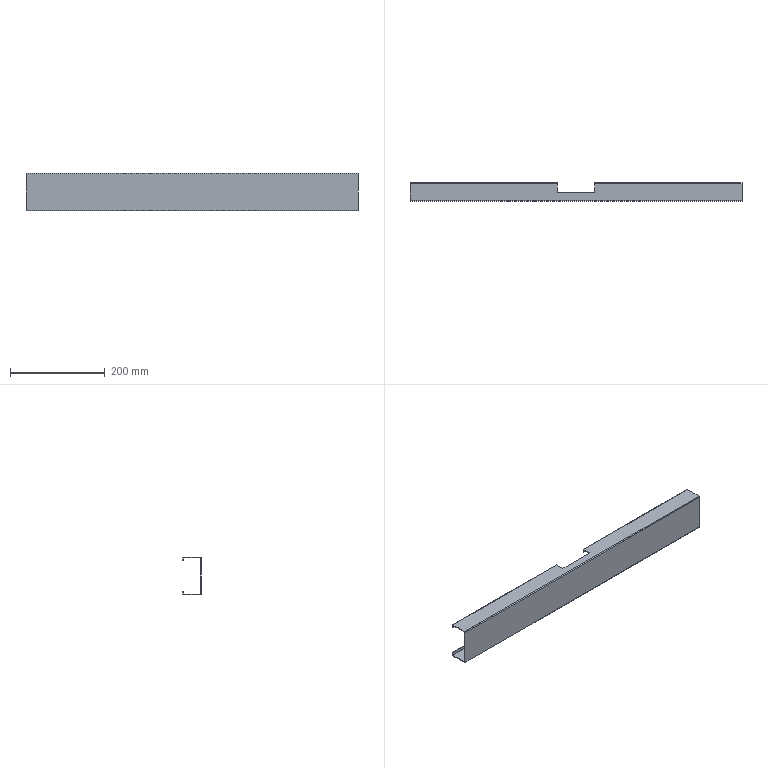Part | SolidWorks | features FlatPattern 1, ICE 1, SMBaseFlange 1, SheetMetal 1 | 1 solid | 62 faces | box 700 x 38 x 80 mm | volume 166325 mm3 | plane 50 | cylinder 12 | commonest cylinder face diameters 0.4 x6 3.4 x6
STEP:
#1=CARTESIAN_POINT('',(-40.,38.,38.3));
#2=VERTEX_POINT('',#1);
#3=CARTESIAN_POINT('',(-40.,38.,32.));
#4=VERTEX_POINT('',#3);
#5=CARTESIAN_POINT('',(-40.,38.,32.));
#6=DIRECTION('',(0.,0.,-1.));
#7=VECTOR('',#6,1000.);
#8=LINE('',#5,#7);
#9=EDGE_CURVE('',#2,#4,#8,.T.);
#10=ORIENTED_EDGE('',*,*,#9,.F.);
#11=CARTESIAN_POINT('',(-40.,36.5,38.3));
#12=VERTEX_POINT('',#11);
#13=CARTESIAN_POINT('',(-40.,38.,38.3));
#14=DIRECTION('',(0.,-1.,0.));
#15=VECTOR('',#14,1000.);
#16=LINE('',#13,#15);
#17=EDGE_CURVE('',#2,#12,#16,.T.);
#18=ORIENTED_EDGE('',*,*,#17,.T.);
#19=CARTESIAN_POINT('',(-40.,36.5,32.));
#20=VERTEX_POINT('',#19);
#21=CARTESIAN_POINT('',(-40.,36.5,32.));
#22=DIRECTION('',(0.,0.,-1.));
#23=VECTOR('',#22,1000.);
#24=LINE('',#21,#23);
#25=EDGE_CURVE('',#12,#20,#24,.T.);
#26=ORIENTED_EDGE('',*,*,#25,.T.);
#27=CARTESIAN_POINT('',(-40.,38.,32.));
#28=DIRECTION('',(0.,1.,0.));
#29=VECTOR('',#28,1000.);
#30=LINE('',#27,#29);
#31=EDGE_CURVE('',#20,#4,#30,.T.);
#32=ORIENTED_EDGE('',*,*,#31,.T.);
#33=EDGE_LOOP('',(#10,#18,#26,#32));
#34=FACE_OUTER_BOUND('',#33,.T.);
#35=CARTESIAN_POINT('',(-40.,58.,-40.));
#36=DIRECTION('',(-1.,0.,0.));
#37=DIRECTION('',(0.,0.,1.));
#38=AXIS2_PLACEMENT_3D('',#35,#36,#37);
#39=PLANE('',#38);
#40=ADVANCED_FACE('',(#34),#39,.F.);
#41=CARTESIAN_POINT('',(-40.,18.,38.5));
#42=VERTEX_POINT('',#41);
#43=CARTESIAN_POINT('',(-40.,36.3,38.5));
#44=VERTEX_POINT('',#43);
#45=CARTESIAN_POINT('',(-40.,38.,38.5));
#46=DIRECTION('',(0.,1.,0.));
#47=VECTOR('',#46,1000.);
#48=LINE('',#45,#47);
#49=EDGE_CURVE('',#42,#44,#48,.T.);
#50=ORIENTED_EDGE('',*,*,#49,.T.);
#51=CARTESIAN_POINT('',(-40.,36.3,40.));
#52=VERTEX_POINT('',#51);
#53=CARTESIAN_POINT('',(-40.,36.3,38.5));
#54=DIRECTION('',(0.,0.,1.));
#55=VECTOR('',#54,1000.);
#56=LINE('',#53,#55);
#57=EDGE_CURVE('',#44,#52,#56,.T.);
#58=ORIENTED_EDGE('',*,*,#57,.T.);
#59=CARTESIAN_POINT('',(-40.,18.,40.));
#60=VERTEX_POINT('',#59);
#61=CARTESIAN_POINT('',(-40.,38.,40.));
#62=DIRECTION('',(0.,1.,0.));
#63=VECTOR('',#62,1000.);
#64=LINE('',#61,#63);
#65=EDGE_CURVE('',#60,#52,#64,.T.);
#66=ORIENTED_EDGE('',*,*,#65,.F.);
#67=CARTESIAN_POINT('',(-40.,18.,-40.));
#68=DIRECTION('',(0.,0.,1.));
#69=VECTOR('',#68,1000.);
#70=LINE('',#67,#69);
#71=EDGE_CURVE('',#42,#60,#70,.T.);
#72=ORIENTED_EDGE('',*,*,#71,.F.);
#73=EDGE_LOOP('',(#50,#58,#66,#72));
#74=FACE_OUTER_BOUND('',#73,.T.);
#75=CARTESIAN_POINT('',(-40.,58.,-40.));
#76=DIRECTION('',(-1.,0.,0.));
#77=DIRECTION('',(0.,0.,1.));
#78=AXIS2_PLACEMENT_3D('',#75,#76,#77);
#79=PLANE('',#78);
#80=ADVANCED_FACE('',(#74),#79,.F.);
#81=CARTESIAN_POINT('',(40.,36.5,32.));
#82=VERTEX_POINT('',#81);
#83=CARTESIAN_POINT('',(40.,36.5,38.3));
#84=VERTEX_POINT('',#83);
#85=CARTESIAN_POINT('',(40.,36.5,32.));
#86=DIRECTION('',(0.,0.,1.));
#87=VECTOR('',#86,1000.);
#88=LINE('',#85,#87);
#89=EDGE_CURVE('',#82,#84,#88,.T.);
#90=ORIENTED_EDGE('',*,*,#89,.T.);
#91=CARTESIAN_POINT('',(40.,38.,38.3));
#92=VERTEX_POINT('',#91);
#93=CARTESIAN_POINT('',(40.,36.5,38.3));
#94=DIRECTION('',(0.,1.,0.));
#95=VECTOR('',#94,1000.);
#96=LINE('',#93,#95);
#97=EDGE_CURVE('',#84,#92,#96,.T.);
#98=ORIENTED_EDGE('',*,*,#97,.T.);
#99=CARTESIAN_POINT('',(40.,38.,32.));
#100=VERTEX_POINT('',#99);
#101=CARTESIAN_POINT('',(40.,38.,32.));
#102=DIRECTION('',(0.,0.,1.));
#103=VECTOR('',#102,1000.);
#104=LINE('',#101,#103);
#105=EDGE_CURVE('',#100,#92,#104,.T.);
#106=ORIENTED_EDGE('',*,*,#105,.F.);
#107=CARTESIAN_POINT('',(40.,38.,32.));
#108=DIRECTION('',(0.,-1.,0.));
#109=VECTOR('',#108,1000.);
#110=LINE('',#107,#109);
#111=EDGE_CURVE('',#100,#82,#110,.T.);
#112=ORIENTED_EDGE('',*,*,#111,.T.);
#113=EDGE_LOOP('',(#90,#98,#106,#112));
#114=FACE_OUTER_BOUND('',#113,.T.);
#115=CARTESIAN_POINT('',(40.,58.,-40.));
#116=DIRECTION('',(1.,0.,0.));
#117=DIRECTION('',(0.,0.,-1.));
#118=AXIS2_PLACEMENT_3D('',#115,#116,#117);
#119=PLANE('',#118);
#120=ADVANCED_FACE('',(#114),#119,.F.);
#121=CARTESIAN_POINT('',(40.,36.3,40.));
#122=VERTEX_POINT('',#121);
#123=CARTESIAN_POINT('',(40.,18.,40.));
#124=VERTEX_POINT('',#123);
#125=CARTESIAN_POINT('',(40.,38.,40.));
#126=DIRECTION('',(0.,-1.,0.));
#127=VECTOR('',#126,1000.);
#128=LINE('',#125,#127);
#129=EDGE_CURVE('',#122,#124,#128,.T.);
#130=ORIENTED_EDGE('',*,*,#129,.F.);
#131=CARTESIAN_POINT('',(40.,36.3,38.5));
#132=VERTEX_POINT('',#131);
#133=CARTESIAN_POINT('',(40.,36.3,40.));
#134=DIRECTION('',(0.,0.,-1.));
#135=VECTOR('',#134,1000.);
#136=LINE('',#133,#135);
#137=EDGE_CURVE('',#122,#132,#136,.T.);
#138=ORIENTED_EDGE('',*,*,#137,.T.);
#139=CARTESIAN_POINT('',(40.,18.,38.5));
#140=VERTEX_POINT('',#139);
#141=CARTESIAN_POINT('',(40.,38.,38.5));
#142=DIRECTION('',(0.,-1.,0.));
#143=VECTOR('',#142,1000.);
#144=LINE('',#141,#143);
#145=EDGE_CURVE('',#132,#140,#144,.T.);
#146=ORIENTED_EDGE('',*,*,#145,.T.);
#147=CARTESIAN_POINT('',(40.,18.,-40.));
#148=DIRECTION('',(0.,0.,1.));
#149=VECTOR('',#148,1000.);
#150=LINE('',#147,#149);
#151=EDGE_CURVE('',#140,#124,#150,.T.);
#152=ORIENTED_EDGE('',*,*,#151,.T.);
#153=EDGE_LOOP('',(#130,#138,#146,#152));
#154=FACE_OUTER_BOUND('',#153,.T.);
#155=CARTESIAN_POINT('',(40.,58.,-40.));
#156=DIRECTION('',(1.,0.,0.));
#157=DIRECTION('',(0.,0.,-1.));
#158=AXIS2_PLACEMENT_3D('',#155,#156,#157);
#159=PLANE('',#158);
#160=ADVANCED_FACE('',(#154),#159,.F.);
#161=CARTESIAN_POINT('',(-40.,36.5,-32.));
#162=VERTEX_POINT('',#161);
#163=CARTESIAN_POINT('',(-40.,36.5,-38.3));
#164=VERTEX_POINT('',#163);
#165=CARTESIAN_POINT('',(-40.,36.5,-40.));
#166=DIRECTION('',(0.,0.,-1.));
#167=VECTOR('',#166,1000.);
#168=LINE('',#165,#167);
#169=EDGE_CURVE('',#162,#164,#168,.T.);
#170=ORIENTED_EDGE('',*,*,#169,.T.);
#171=CARTESIAN_POINT('',(-40.,38.,-38.3));
#172=VERTEX_POINT('',#171);
#173=CARTESIAN_POINT('',(-40.,36.5,-38.3));
#174=DIRECTION('',(0.,1.,0.));
#175=VECTOR('',#174,1000.);
#176=LINE('',#173,#175);
#177=EDGE_CURVE('',#164,#172,#176,.T.);
#178=ORIENTED_EDGE('',*,*,#177,.T.);
#179=CARTESIAN_POINT('',(-40.,38.,-32.));
#180=VERTEX_POINT('',#179);
#181=CARTESIAN_POINT('',(-40.,38.,-40.));
#182=DIRECTION('',(0.,0.,-1.));
#183=VECTOR('',#182,1000.);
#184=LINE('',#181,#183);
#185=EDGE_CURVE('',#180,#172,#184,.T.);
#186=ORIENTED_EDGE('',*,*,#185,.F.);
#187=CARTESIAN_POINT('',(-40.,36.5,-32.));
#188=DIRECTION('',(0.,-1.,0.));
#189=VECTOR('',#188,1000.);
#190=LINE('',#187,#189);
#191=EDGE_CURVE('',#180,#162,#190,.T.);
#192=ORIENTED_EDGE('',*,*,#191,.T.);
#193=EDGE_LOOP('',(#170,#178,#186,#192));
#194=FACE_OUTER_BOUND('',#193,.T.);
#195=CARTESIAN_POINT('',(-40.,58.,-40.));
#196=DIRECTION('',(-1.,0.,0.));
#197=DIRECTION('',(0.,0.,1.));
#198=AXIS2_PLACEMENT_3D('',#195,#196,#197);
#199=PLANE('',#198);
#200=ADVANCED_FACE('',(#194),#199,.F.);
#201=CARTESIAN_POINT('',(-40.,36.3,-40.));
#202=VERTEX_POINT('',#201);
#203=CARTESIAN_POINT('',(-40.,18.,-40.));
#204=VERTEX_POINT('',#203);
#205=CARTESIAN_POINT('',(-40.,58.,-40.));
#206=DIRECTION('',(0.,-1.,0.));
#207=VECTOR('',#206,1000.);
#208=LINE('',#205,#207);
#209=EDGE_CURVE('',#202,#204,#208,.T.);
#210=ORIENTED_EDGE('',*,*,#209,.F.);
#211=CARTESIAN_POINT('',(-40.,36.3,-38.5));
#212=VERTEX_POINT('',#211);
#213=CARTESIAN_POINT('',(-40.,36.3,-40.));
#214=DIRECTION('',(0.,0.,1.));
#215=VECTOR('',#214,1000.);
#216=LINE('',#213,#215);
#217=EDGE_CURVE('',#202,#212,#216,.T.);
#218=ORIENTED_EDGE('',*,*,#217,.T.);
#219=CARTESIAN_POINT('',(-40.,18.,-38.5));
#220=VERTEX_POINT('',#219);
#221=CARTESIAN_POINT('',(-40.,0.,-38.5));
#222=DIRECTION('',(0.,-1.,0.));
#223=VECTOR('',#222,1000.);
#224=LINE('',#221,#223);
#225=EDGE_CURVE('',#212,#220,#224,.T.);
#226=ORIENTED_EDGE('',*,*,#225,.T.);
#227=CARTESIAN_POINT('',(-40.,18.,-40.));
#228=DIRECTION('',(0.,0.,1.));
#229=VECTOR('',#228,1000.);
#230=LINE('',#227,#229);
#231=EDGE_CURVE('',#204,#220,#230,.T.);
#232=ORIENTED_EDGE('',*,*,#231,.F.);
#233=EDGE_LOOP('',(#210,#218,#226,#232));
#234=FACE_OUTER_BOUND('',#233,.T.);
#235=CARTESIAN_POINT('',(-40.,58.,-40.));
#236=DIRECTION('',(-1.,0.,0.));
#237=DIRECTION('',(0.,0.,1.));
#238=AXIS2_PLACEMENT_3D('',#235,#236,#237);
#239=PLANE('',#238);
#240=ADVANCED_FACE('',(#234),#239,.F.);
#241=CARTESIAN_POINT('',(40.,38.,-38.3));
#242=VERTEX_POINT('',#241);
#243=CARTESIAN_POINT('',(40.,38.,-32.));
#244=VERTEX_POINT('',#243);
#245=CARTESIAN_POINT('',(40.,38.,-40.));
#246=DIRECTION('',(0.,0.,1.));
#247=VECTOR('',#246,1000.);
#248=LINE('',#245,#247);
#249=EDGE_CURVE('',#242,#244,#248,.T.);
#250=ORIENTED_EDGE('',*,*,#249,.F.);
#251=CARTESIAN_POINT('',(40.,36.5,-38.3));
#252=VERTEX_POINT('',#251);
#253=CARTESIAN_POINT('',(40.,38.,-38.3));
#254=DIRECTION('',(0.,-1.,0.));
#255=VECTOR('',#254,1000.);
#256=LINE('',#253,#255);
#257=EDGE_CURVE('',#242,#252,#256,.T.);
#258=ORIENTED_EDGE('',*,*,#257,.T.);
#259=CARTESIAN_POINT('',(40.,36.5,-32.));
#260=VERTEX_POINT('',#259);
#261=CARTESIAN_POINT('',(40.,36.5,-40.));
#262=DIRECTION('',(0.,0.,1.));
#263=VECTOR('',#262,1000.);
#264=LINE('',#261,#263);
#265=EDGE_CURVE('',#252,#260,#264,.T.);
#266=ORIENTED_EDGE('',*,*,#265,.T.);
#267=CARTESIAN_POINT('',(40.,36.5,-32.));
#268=DIRECTION('',(0.,1.,0.));
#269=VECTOR('',#268,1000.);
#270=LINE('',#267,#269);
#271=EDGE_CURVE('',#260,#244,#270,.T.);
#272=ORIENTED_EDGE('',*,*,#271,.T.);
#273=EDGE_LOOP('',(#250,#258,#266,#272));
#274=FACE_OUTER_BOUND('',#273,.T.);
#275=CARTESIAN_POINT('',(40.,58.,-40.));
#276=DIRECTION('',(1.,0.,0.));
#277=DIRECTION('',(0.,0.,-1.));
#278=AXIS2_PLACEMENT_3D('',#275,#276,#277);
#279=PLANE('',#278);
#280=ADVANCED_FACE('',(#274),#279,.F.);
#281=CARTESIAN_POINT('',(40.,18.,-38.5));
#282=VERTEX_POINT('',#281);
#283=CARTESIAN_POINT('',(40.,36.3,-38.5));
#284=VERTEX_POINT('',#283);
#285=CARTESIAN_POINT('',(40.,0.,-38.5));
#286=DIRECTION('',(0.,1.,0.));
#287=VECTOR('',#286,1000.);
#288=LINE('',#285,#287);
#289=EDGE_CURVE('',#282,#284,#288,.T.);
#290=ORIENTED_EDGE('',*,*,#289,.T.);
#291=CARTESIAN_POINT('',(40.,36.3,-40.));
#292=VERTEX_POINT('',#291);
#293=CARTESIAN_POINT('',(40.,36.3,-38.5));
#294=DIRECTION('',(0.,0.,-1.));
#295=VECTOR('',#294,1000.);
#296=LINE('',#293,#295);
#297=EDGE_CURVE('',#284,#292,#296,.T.);
#298=ORIENTED_EDGE('',*,*,#297,.T.);
#299=CARTESIAN_POINT('',(40.,18.,-40.));
#300=VERTEX_POINT('',#299);
#301=CARTESIAN_POINT('',(40.,58.,-40.));
#302=DIRECTION('',(0.,1.,0.));
#303=VECTOR('',#302,1000.);
#304=LINE('',#301,#303);
#305=EDGE_CURVE('',#300,#292,#304,.T.);
#306=ORIENTED_EDGE('',*,*,#305,.F.);
#307=CARTESIAN_POINT('',(40.,18.,-40.));
#308=DIRECTION('',(0.,0.,1.));
#309=VECTOR('',#308,1000.);
#310=LINE('',#307,#309);
#311=EDGE_CURVE('',#300,#282,#310,.T.);
#312=ORIENTED_EDGE('',*,*,#311,.T.);
#313=EDGE_LOOP('',(#290,#298,#306,#312));
#314=FACE_OUTER_BOUND('',#313,.T.);
#315=CARTESIAN_POINT('',(40.,58.,-40.));
#316=DIRECTION('',(1.,0.,0.));
#317=DIRECTION('',(0.,0.,-1.));
#318=AXIS2_PLACEMENT_3D('',#315,#316,#317);
#319=PLANE('',#318);
#320=ADVANCED_FACE('',(#314),#319,.F.);
#321=CARTESIAN_POINT('',(350.,38.,-38.3));
#322=VERTEX_POINT('',#321);
#323=CARTESIAN_POINT('',(350.,38.,-38.3));
#324=DIRECTION('',(-1.,0.,0.));
#325=VECTOR('',#324,1000.);
#326=LINE('',#323,#325);
#327=EDGE_CURVE('',#322,#242,#326,.T.);
#328=ORIENTED_EDGE('',*,*,#327,.T.);
#329=ORIENTED_EDGE('',*,*,#249,.T.);
#330=CARTESIAN_POINT('',(350.,38.,-32.));
#331=VERTEX_POINT('',#330);
#332=CARTESIAN_POINT('',(350.,38.,-32.));
#333=DIRECTION('',(-1.,0.,0.));
#334=VECTOR('',#333,1000.);
#335=LINE('',#332,#334);
#336=EDGE_CURVE('',#331,#244,#335,.T.);
#337=ORIENTED_EDGE('',*,*,#336,.F.);
#338=CARTESIAN_POINT('',(350.,38.,-40.));
#339=DIRECTION('',(0.,0.,1.));
#340=VECTOR('',#339,1000.);
#341=LINE('',#338,#340);
#342=EDGE_CURVE('',#322,#331,#341,.T.);
#343=ORIENTED_EDGE('',*,*,#342,.F.);
#344=EDGE_LOOP('',(#328,#329,#337,#343));
#345=FACE_OUTER_BOUND('',#344,.T.);
#346=CARTESIAN_POINT('',(350.,38.,-40.));
#347=DIRECTION('',(0.,-1.,0.));
#348=DIRECTION('',(0.,0.,-1.));
#349=AXIS2_PLACEMENT_3D('',#346,#347,#348);
#350=PLANE('',#349);
#351=ADVANCED_FACE('',(#345),#350,.F.);
#352=ORIENTED_EDGE('',*,*,#271,.F.);
#353=CARTESIAN_POINT('',(350.,36.5,-32.));
#354=VERTEX_POINT('',#353);
#355=CARTESIAN_POINT('',(350.,36.5,-32.));
#356=DIRECTION('',(-1.,0.,0.));
#357=VECTOR('',#356,1000.);
#358=LINE('',#355,#357);
#359=EDGE_CURVE('',#354,#260,#358,.T.);
#360=ORIENTED_EDGE('',*,*,#359,.F.);
#361=CARTESIAN_POINT('',(350.,36.5,-32.));
#362=DIRECTION('',(0.,1.,0.));
#363=VECTOR('',#362,1000.);
#364=LINE('',#361,#363);
#365=EDGE_CURVE('',#354,#331,#364,.T.);
#366=ORIENTED_EDGE('',*,*,#365,.T.);
#367=ORIENTED_EDGE('',*,*,#336,.T.);
#368=EDGE_LOOP('',(#352,#360,#366,#367));
#369=FACE_OUTER_BOUND('',#368,.T.);
#370=CARTESIAN_POINT('',(350.,36.5,-32.));
#371=DIRECTION('',(0.,0.,1.));
#372=DIRECTION('',(1.,0.,0.));
#373=AXIS2_PLACEMENT_3D('',#370,#371,#372);
#374=PLANE('',#373);
#375=ADVANCED_FACE('',(#369),#374,.T.);
#376=ORIENTED_EDGE('',*,*,#265,.F.);
#377=CARTESIAN_POINT('',(350.,36.5,-38.3));
#378=VERTEX_POINT('',#377);
#379=CARTESIAN_POINT('',(350.,36.5,-38.3));
#380=DIRECTION('',(-1.,0.,0.));
#381=VECTOR('',#380,1000.);
#382=LINE('',#379,#381);
#383=EDGE_CURVE('',#378,#252,#382,.T.);
#384=ORIENTED_EDGE('',*,*,#383,.F.);
#385=CARTESIAN_POINT('',(350.,36.5,-40.));
#386=DIRECTION('',(0.,0.,1.));
#387=VECTOR('',#386,1000.);
#388=LINE('',#385,#387);
#389=EDGE_CURVE('',#378,#354,#388,.T.);
#390=ORIENTED_EDGE('',*,*,#389,.T.);
#391=ORIENTED_EDGE('',*,*,#359,.T.);
#392=EDGE_LOOP('',(#376,#384,#390,#391));
#393=FACE_OUTER_BOUND('',#392,.T.);
#394=CARTESIAN_POINT('',(350.,36.5,-40.));
#395=DIRECTION('',(0.,-1.,0.));
#396=DIRECTION('',(0.,0.,-1.));
#397=AXIS2_PLACEMENT_3D('',#394,#395,#396);
#398=PLANE('',#397);
#399=ADVANCED_FACE('',(#393),#398,.T.);
#400=CARTESIAN_POINT('',(40.,36.3,-38.3));
#401=DIRECTION('',(1.,0.,0.));
#402=DIRECTION('',(0.,0.,-1.));
#403=AXIS2_PLACEMENT_3D('',#400,#401,#402);
#404=CIRCLE('',#403,0.2);
#405=EDGE_CURVE('',#284,#252,#404,.T.);
#406=ORIENTED_EDGE('',*,*,#405,.F.);
#407=CARTESIAN_POINT('',(350.,36.3,-38.5));
#408=VERTEX_POINT('',#407);
#409=CARTESIAN_POINT('',(350.,36.3,-38.5));
#410=DIRECTION('',(-1.,0.,0.));
#411=VECTOR('',#410,1000.);
#412=LINE('',#409,#411);
#413=EDGE_CURVE('',#408,#284,#412,.T.);
#414=ORIENTED_EDGE('',*,*,#413,.F.);
#415=CARTESIAN_POINT('',(350.,36.3,-38.3));
#416=DIRECTION('',(1.,0.,0.));
#417=DIRECTION('',(0.,0.,-1.));
#418=AXIS2_PLACEMENT_3D('',#415,#416,#417);
#419=CIRCLE('',#418,0.2);
#420=EDGE_CURVE('',#408,#378,#419,.T.);
#421=ORIENTED_EDGE('',*,*,#420,.T.);
#422=ORIENTED_EDGE('',*,*,#383,.T.);
#423=EDGE_LOOP('',(#406,#414,#421,#422));
#424=FACE_OUTER_BOUND('',#423,.T.);
#425=CARTESIAN_POINT('',(350.,36.3,-38.3));
#426=DIRECTION('',(-1.,0.,0.));
#427=DIRECTION('',(0.,0.,1.));
#428=AXIS2_PLACEMENT_3D('',#425,#426,#427);
#429=CYLINDRICAL_SURFACE('',#428,0.2);
#430=ADVANCED_FACE('',(#424),#429,.F.);
#431=CARTESIAN_POINT('',(40.,36.3,38.3));
#432=DIRECTION('',(1.,0.,0.));
#433=DIRECTION('',(0.,0.,-1.));
#434=AXIS2_PLACEMENT_3D('',#431,#432,#433);
#435=CIRCLE('',#434,0.2);
#436=EDGE_CURVE('',#84,#132,#435,.T.);
#437=ORIENTED_EDGE('',*,*,#436,.F.);
#438=CARTESIAN_POINT('',(350.,36.5,38.3));
#439=VERTEX_POINT('',#438);
#440=CARTESIAN_POINT('',(350.,36.5,38.3));
#441=DIRECTION('',(-1.,0.,0.));
#442=VECTOR('',#441,1000.);
#443=LINE('',#440,#442);
#444=EDGE_CURVE('',#439,#84,#443,.T.);
#445=ORIENTED_EDGE('',*,*,#444,.F.);
#446=CARTESIAN_POINT('',(350.,36.3,38.5));
#447=VERTEX_POINT('',#446);
#448=CARTESIAN_POINT('',(350.,36.3,38.3));
#449=DIRECTION('',(1.,0.,0.));
#450=DIRECTION('',(0.,0.,-1.));
#451=AXIS2_PLACEMENT_3D('',#448,#449,#450);
#452=CIRCLE('',#451,0.2);
#453=EDGE_CURVE('',#439,#447,#452,.T.);
#454=ORIENTED_EDGE('',*,*,#453,.T.);
#455=CARTESIAN_POINT('',(350.,36.3,38.5));
#456=DIRECTION('',(-1.,0.,0.));
#457=VECTOR('',#456,1000.);
#458=LINE('',#455,#457);
#459=EDGE_CURVE('',#447,#132,#458,.T.);
#460=ORIENTED_EDGE('',*,*,#459,.T.);
#461=EDGE_LOOP('',(#437,#445,#454,#460));
#462=FACE_OUTER_BOUND('',#461,.T.);
#463=CARTESIAN_POINT('',(350.,36.3,38.3));
#464=DIRECTION('',(-1.,0.,0.));
#465=DIRECTION('',(0.,0.,1.));
#466=AXIS2_PLACEMENT_3D('',#463,#464,#465);
#467=CYLINDRICAL_SURFACE('',#466,0.2);
#468=ADVANCED_FACE('',(#462),#467,.F.);
#469=ORIENTED_EDGE('',*,*,#89,.F.);
#470=CARTESIAN_POINT('',(350.,36.5,32.));
#471=VERTEX_POINT('',#470);
#472=CARTESIAN_POINT('',(350.,36.5,32.));
#473=DIRECTION('',(-1.,0.,0.));
#474=VECTOR('',#473,1000.);
#475=LINE('',#472,#474);
#476=EDGE_CURVE('',#471,#82,#475,.T.);
#477=ORIENTED_EDGE('',*,*,#476,.F.);
#478=CARTESIAN_POINT('',(350.,36.5,32.));
#479=DIRECTION('',(0.,0.,1.));
#480=VECTOR('',#479,1000.);
#481=LINE('',#478,#480);
#482=EDGE_CURVE('',#471,#439,#481,.T.);
#483=ORIENTED_EDGE('',*,*,#482,.T.);
#484=ORIENTED_EDGE('',*,*,#444,.T.);
#485=EDGE_LOOP('',(#469,#477,#483,#484));
#486=FACE_OUTER_BOUND('',#485,.T.);
#487=CARTESIAN_POINT('',(350.,36.5,32.));
#488=DIRECTION('',(0.,-1.,0.));
#489=DIRECTION('',(0.,0.,-1.));
#490=AXIS2_PLACEMENT_3D('',#487,#488,#489);
#491=PLANE('',#490);
#492=ADVANCED_FACE('',(#486),#491,.T.);
#493=ORIENTED_EDGE('',*,*,#111,.F.);
#494=CARTESIAN_POINT('',(350.,38.,32.));
#495=VERTEX_POINT('',#494);
#496=CARTESIAN_POINT('',(350.,38.,32.));
#497=DIRECTION('',(-1.,0.,0.));
#498=VECTOR('',#497,1000.);
#499=LINE('',#496,#498);
#500=EDGE_CURVE('',#495,#100,#499,.T.);
#501=ORIENTED_EDGE('',*,*,#500,.F.);
#502=CARTESIAN_POINT('',(350.,38.,32.));
#503=DIRECTION('',(0.,-1.,0.));
#504=VECTOR('',#503,1000.);
#505=LINE('',#502,#504);
#506=EDGE_CURVE('',#495,#471,#505,.T.);
#507=ORIENTED_EDGE('',*,*,#506,.T.);
#508=ORIENTED_EDGE('',*,*,#476,.T.);
#509=EDGE_LOOP('',(#493,#501,#507,#508));
#510=FACE_OUTER_BOUND('',#509,.T.);
#511=CARTESIAN_POINT('',(350.,38.,32.));
#512=DIRECTION('',(0.,0.,-1.));
#513=DIRECTION('',(-1.,0.,0.));
#514=AXIS2_PLACEMENT_3D('',#511,#512,#513);
#515=PLANE('',#514);
#516=ADVANCED_FACE('',(#510),#515,.T.);
#517=ORIENTED_EDGE('',*,*,#500,.T.);
#518=ORIENTED_EDGE('',*,*,#105,.T.);
#519=CARTESIAN_POINT('',(350.,38.,38.3));
#520=VERTEX_POINT('',#519);
#521=CARTESIAN_POINT('',(350.,38.,38.3));
#522=DIRECTION('',(-1.,0.,0.));
#523=VECTOR('',#522,1000.);
#524=LINE('',#521,#523);
#525=EDGE_CURVE('',#520,#92,#524,.T.);
#526=ORIENTED_EDGE('',*,*,#525,.F.);
#527=CARTESIAN_POINT('',(350.,38.,32.));
#528=DIRECTION('',(0.,0.,1.));
#529=VECTOR('',#528,1000.);
#530=LINE('',#527,#529);
#531=EDGE_CURVE('',#495,#520,#530,.T.);
#532=ORIENTED_EDGE('',*,*,#531,.F.);
#533=EDGE_LOOP('',(#517,#518,#526,#532));
#534=FACE_OUTER_BOUND('',#533,.T.);
#535=CARTESIAN_POINT('',(350.,38.,32.));
#536=DIRECTION('',(0.,-1.,0.));
#537=DIRECTION('',(0.,0.,-1.));
#538=AXIS2_PLACEMENT_3D('',#535,#536,#537);
#539=PLANE('',#538);
#540=ADVANCED_FACE('',(#534),#539,.F.);
#541=ORIENTED_EDGE('',*,*,#525,.T.);
#542=CARTESIAN_POINT('',(40.,36.3,38.3));
#543=DIRECTION('',(1.,0.,0.));
#544=DIRECTION('',(0.,0.,-1.));
#545=AXIS2_PLACEMENT_3D('',#542,#543,#544);
#546=CIRCLE('',#545,1.7);
#547=EDGE_CURVE('',#92,#122,#546,.T.);
#548=ORIENTED_EDGE('',*,*,#547,.T.);
#549=CARTESIAN_POINT('',(350.,36.3,40.));
#550=VERTEX_POINT('',#549);
#551=CARTESIAN_POINT('',(350.,36.3,40.));
#552=DIRECTION('',(-1.,0.,0.));
#553=VECTOR('',#552,1000.);
#554=LINE('',#551,#553);
#555=EDGE_CURVE('',#550,#122,#554,.T.);
#556=ORIENTED_EDGE('',*,*,#555,.F.);
#557=CARTESIAN_POINT('',(350.,36.3,38.3));
#558=DIRECTION('',(1.,0.,0.));
#559=DIRECTION('',(0.,0.,1.));
#560=AXIS2_PLACEMENT_3D('',#557,#558,#559);
#561=CIRCLE('',#560,1.7);
#562=EDGE_CURVE('',#520,#550,#561,.T.);
#563=ORIENTED_EDGE('',*,*,#562,.F.);
#564=EDGE_LOOP('',(#541,#548,#556,#563));
#565=FACE_OUTER_BOUND('',#564,.T.);
#566=CARTESIAN_POINT('',(350.,36.3,38.3));
#567=DIRECTION('',(-1.,0.,0.));
#568=DIRECTION('',(0.,0.,1.));
#569=AXIS2_PLACEMENT_3D('',#566,#567,#568);
#570=CYLINDRICAL_SURFACE('',#569,1.7);
#571=ADVANCED_FACE('',(#565),#570,.T.);
#572=CARTESIAN_POINT('',(350.,36.3,-40.));
#573=VERTEX_POINT('',#572);
#574=CARTESIAN_POINT('',(350.,36.3,-40.));
#575=DIRECTION('',(-1.,0.,0.));
#576=VECTOR('',#575,1000.);
#577=LINE('',#574,#576);
#578=EDGE_CURVE('',#573,#292,#577,.T.);
#579=ORIENTED_EDGE('',*,*,#578,.T.);
#580=CARTESIAN_POINT('',(40.,36.3,-38.3));
#581=DIRECTION('',(1.,0.,0.));
#582=DIRECTION('',(0.,0.,-1.));
#583=AXIS2_PLACEMENT_3D('',#580,#581,#582);
#584=CIRCLE('',#583,1.7);
#585=EDGE_CURVE('',#292,#242,#584,.T.);
#586=ORIENTED_EDGE('',*,*,#585,.T.);
#587=ORIENTED_EDGE('',*,*,#327,.F.);
#588=CARTESIAN_POINT('',(350.,36.3,-38.3));
#589=DIRECTION('',(1.,0.,0.));
#590=DIRECTION('',(0.,0.,1.));
#591=AXIS2_PLACEMENT_3D('',#588,#589,#590);
#592=CIRCLE('',#591,1.7);
#593=EDGE_CURVE('',#573,#322,#592,.T.);
#594=ORIENTED_EDGE('',*,*,#593,.F.);
#595=EDGE_LOOP('',(#579,#586,#587,#594));
#596=FACE_OUTER_BOUND('',#595,.T.);
#597=CARTESIAN_POINT('',(350.,36.3,-38.3));
#598=DIRECTION('',(-1.,0.,0.));
#599=DIRECTION('',(0.,0.,1.));
#600=AXIS2_PLACEMENT_3D('',#597,#598,#599);
#601=CYLINDRICAL_SURFACE('',#600,1.7);
#602=ADVANCED_FACE('',(#596),#601,.T.);
#603=CARTESIAN_POINT('',(350.,38.,38.3));
#604=DIRECTION('',(0.,-1.,0.));
#605=VECTOR('',#604,1000.);
#606=LINE('',#603,#605);
#607=EDGE_CURVE('',#520,#439,#606,.T.);
#608=ORIENTED_EDGE('',*,*,#607,.F.);
#609=ORIENTED_EDGE('',*,*,#562,.T.);
#610=CARTESIAN_POINT('',(350.,36.3,38.5));
#611=DIRECTION('',(0.,0.,1.));
#612=VECTOR('',#611,1000.);
#613=LINE('',#610,#612);
#614=EDGE_CURVE('',#447,#550,#613,.T.);
#615=ORIENTED_EDGE('',*,*,#614,.F.);
#616=ORIENTED_EDGE('',*,*,#453,.F.);
#617=EDGE_LOOP('',(#608,#609,#615,#616));
#618=FACE_OUTER_BOUND('',#617,.T.);
#619=CARTESIAN_POINT('',(350.,38.,38.3));
#620=DIRECTION('',(1.,0.,0.));
#621=DIRECTION('',(0.,0.,-1.));
#622=AXIS2_PLACEMENT_3D('',#619,#620,#621);
#623=PLANE('',#622);
#624=ADVANCED_FACE('',(#618),#623,.T.);
#625=ORIENTED_EDGE('',*,*,#531,.T.);
#626=ORIENTED_EDGE('',*,*,#607,.T.);
#627=ORIENTED_EDGE('',*,*,#482,.F.);
#628=ORIENTED_EDGE('',*,*,#506,.F.);
#629=EDGE_LOOP('',(#625,#626,#627,#628));
#630=FACE_OUTER_BOUND('',#629,.T.);
#631=CARTESIAN_POINT('',(350.,36.3,38.5));
#632=DIRECTION('',(1.,0.,0.));
#633=DIRECTION('',(0.,0.,-1.));
#634=AXIS2_PLACEMENT_3D('',#631,#632,#633);
#635=PLANE('',#634);
#636=ADVANCED_FACE('',(#630),#635,.T.);
#637=CARTESIAN_POINT('',(-350.,36.3,40.));
#638=VERTEX_POINT('',#637);
#639=CARTESIAN_POINT('',(-350.,36.3,38.5));
#640=VERTEX_POINT('',#639);
#641=CARTESIAN_POINT('',(-350.,36.3,40.));
#642=DIRECTION('',(0.,0.,-1.));
#643=VECTOR('',#642,1000.);
#644=LINE('',#641,#643);
#645=EDGE_CURVE('',#638,#640,#644,.T.);
#646=ORIENTED_EDGE('',*,*,#645,.F.);
#647=CARTESIAN_POINT('',(-350.,38.,38.3));
#648=VERTEX_POINT('',#647);
#649=CARTESIAN_POINT('',(-350.,36.3,38.3));
#650=DIRECTION('',(1.,0.,0.));
#651=DIRECTION('',(0.,0.,1.));
#652=AXIS2_PLACEMENT_3D('',#649,#650,#651);
#653=CIRCLE('',#652,1.7);
#654=EDGE_CURVE('',#648,#638,#653,.T.);
#655=ORIENTED_EDGE('',*,*,#654,.F.);
#656=CARTESIAN_POINT('',(-350.,36.5,38.3));
#657=VERTEX_POINT('',#656);
#658=CARTESIAN_POINT('',(-350.,36.5,38.3));
#659=DIRECTION('',(0.,1.,0.));
#660=VECTOR('',#659,1000.);
#661=LINE('',#658,#660);
#662=EDGE_CURVE('',#657,#648,#661,.T.);
#663=ORIENTED_EDGE('',*,*,#662,.F.);
#664=CARTESIAN_POINT('',(-350.,36.3,38.3));
#665=DIRECTION('',(1.,0.,0.));
#666=DIRECTION('',(0.,0.,-1.));
#667=AXIS2_PLACEMENT_3D('',#664,#665,#666);
#668=CIRCLE('',#667,0.2);
#669=EDGE_CURVE('',#657,#640,#668,.T.);
#670=ORIENTED_EDGE('',*,*,#669,.T.);
#671=EDGE_LOOP('',(#646,#655,#663,#670));
#672=FACE_OUTER_BOUND('',#671,.T.);
#673=CARTESIAN_POINT('',(-350.,36.3,40.));
#674=DIRECTION('',(-1.,0.,0.));
#675=DIRECTION('',(0.,0.,1.));
#676=AXIS2_PLACEMENT_3D('',#673,#674,#675);
#677=PLANE('',#676);
#678=ADVANCED_FACE('',(#672),#677,.T.);
#679=CARTESIAN_POINT('',(-350.,1.7,40.));
#680=VERTEX_POINT('',#679);
#681=CARTESIAN_POINT('',(-350.,38.,40.));
#682=DIRECTION('',(0.,-1.,0.));
#683=VECTOR('',#682,1000.);
#684=LINE('',#681,#683);
#685=EDGE_CURVE('',#638,#680,#684,.T.);
#686=ORIENTED_EDGE('',*,*,#685,.F.);
#687=ORIENTED_EDGE('',*,*,#645,.T.);
#688=CARTESIAN_POINT('',(-350.,1.7,38.5));
#689=VERTEX_POINT('',#688);
#690=CARTESIAN_POINT('',(-350.,38.,38.5));
#691=DIRECTION('',(0.,-1.,0.));
#692=VECTOR('',#691,1000.);
#693=LINE('',#690,#692);
#694=EDGE_CURVE('',#640,#689,#693,.T.);
#695=ORIENTED_EDGE('',*,*,#694,.T.);
#696=CARTESIAN_POINT('',(-350.,1.7,38.5));
#697=DIRECTION('',(0.,0.,1.));
#698=VECTOR('',#697,1000.);
#699=LINE('',#696,#698);
#700=EDGE_CURVE('',#689,#680,#699,.T.);
#701=ORIENTED_EDGE('',*,*,#700,.T.);
#702=EDGE_LOOP('',(#686,#687,#695,#701));
#703=FACE_OUTER_BOUND('',#702,.T.);
#704=CARTESIAN_POINT('',(-350.,36.5,38.3));
#705=DIRECTION('',(-1.,0.,0.));
#706=DIRECTION('',(0.,0.,1.));
#707=AXIS2_PLACEMENT_3D('',#704,#705,#706);
#708=PLANE('',#707);
#709=ADVANCED_FACE('',(#703),#708,.T.);
#710=CARTESIAN_POINT('',(350.,1.7,40.));
#711=VERTEX_POINT('',#710);
#712=CARTESIAN_POINT('',(350.,1.7,38.5));
#713=VERTEX_POINT('',#712);
#714=CARTESIAN_POINT('',(350.,1.7,40.));
#715=DIRECTION('',(0.,0.,-1.));
#716=VECTOR('',#715,1000.);
#717=LINE('',#714,#716);
#718=EDGE_CURVE('',#711,#713,#717,.T.);
#719=ORIENTED_EDGE('',*,*,#718,.F.);
#720=CARTESIAN_POINT('',(350.,0.,38.3));
#721=VERTEX_POINT('',#720);
#722=CARTESIAN_POINT('',(350.,1.7,38.3));
#723=DIRECTION('',(1.,0.,0.));
#724=DIRECTION('',(0.,0.,1.));
#725=AXIS2_PLACEMENT_3D('',#722,#723,#724);
#726=CIRCLE('',#725,1.7);
#727=EDGE_CURVE('',#711,#721,#726,.T.);
#728=ORIENTED_EDGE('',*,*,#727,.T.);
#729=CARTESIAN_POINT('',(350.,1.5,38.3));
#730=VERTEX_POINT('',#729);
#731=CARTESIAN_POINT('',(350.,1.5,38.3));
#732=DIRECTION('',(0.,-1.,0.));
#733=VECTOR('',#732,1000.);
#734=LINE('',#731,#733);
#735=EDGE_CURVE('',#730,#721,#734,.T.);
#736=ORIENTED_EDGE('',*,*,#735,.F.);
#737=CARTESIAN_POINT('',(350.,1.7,38.3));
#738=DIRECTION('',(1.,0.,0.));
#739=DIRECTION('',(0.,0.,-1.));
#740=AXIS2_PLACEMENT_3D('',#737,#738,#739);
#741=CIRCLE('',#740,0.2);
#742=EDGE_CURVE('',#713,#730,#741,.T.);
#743=ORIENTED_EDGE('',*,*,#742,.F.);
#744=EDGE_LOOP('',(#719,#728,#736,#743));
#745=FACE_OUTER_BOUND('',#744,.T.);
#746=CARTESIAN_POINT('',(350.,1.7,40.));
#747=DIRECTION('',(1.,0.,0.));
#748=DIRECTION('',(0.,0.,-1.));
#749=AXIS2_PLACEMENT_3D('',#746,#747,#748);
#750=PLANE('',#749);
#751=ADVANCED_FACE('',(#745),#750,.T.);
#752=CARTESIAN_POINT('',(350.,38.,40.));
#753=DIRECTION('',(0.,-1.,0.));
#754=VECTOR('',#753,1000.);
#755=LINE('',#752,#754);
#756=EDGE_CURVE('',#550,#711,#755,.T.);
#757=ORIENTED_EDGE('',*,*,#756,.T.);
#758=ORIENTED_EDGE('',*,*,#718,.T.);
#759=CARTESIAN_POINT('',(350.,38.,38.5));
#760=DIRECTION('',(0.,-1.,0.));
#761=VECTOR('',#760,1000.);
#762=LINE('',#759,#761);
#763=EDGE_CURVE('',#447,#713,#762,.T.);
#764=ORIENTED_EDGE('',*,*,#763,.F.);
#765=ORIENTED_EDGE('',*,*,#614,.T.);
#766=EDGE_LOOP('',(#757,#758,#764,#765));
#767=FACE_OUTER_BOUND('',#766,.T.);
#768=CARTESIAN_POINT('',(350.,1.5,38.3));
#769=DIRECTION('',(1.,0.,0.));
#770=DIRECTION('',(0.,0.,-1.));
#771=AXIS2_PLACEMENT_3D('',#768,#769,#770);
#772=PLANE('',#771);
#773=ADVANCED_FACE('',(#767),#772,.T.);
#774=CARTESIAN_POINT('',(-350.,0.,38.3));
#775=VERTEX_POINT('',#774);
#776=CARTESIAN_POINT('',(-350.,1.5,38.3));
#777=VERTEX_POINT('',#776);
#778=CARTESIAN_POINT('',(-350.,0.,38.3));
#779=DIRECTION('',(0.,1.,0.));
#780=VECTOR('',#779,1000.);
#781=LINE('',#778,#780);
#782=EDGE_CURVE('',#775,#777,#781,.T.);
#783=ORIENTED_EDGE('',*,*,#782,.F.);
#784=CARTESIAN_POINT('',(-350.,1.7,38.3));
#785=DIRECTION('',(1.,0.,0.));
#786=DIRECTION('',(0.,0.,1.));
#787=AXIS2_PLACEMENT_3D('',#784,#785,#786);
#788=CIRCLE('',#787,1.7);
#789=EDGE_CURVE('',#680,#775,#788,.T.);
#790=ORIENTED_EDGE('',*,*,#789,.F.);
#791=ORIENTED_EDGE('',*,*,#700,.F.);
#792=CARTESIAN_POINT('',(-350.,1.7,38.3));
#793=DIRECTION('',(1.,0.,0.));
#794=DIRECTION('',(0.,0.,-1.));
#795=AXIS2_PLACEMENT_3D('',#792,#793,#794);
#796=CIRCLE('',#795,0.2);
#797=EDGE_CURVE('',#689,#777,#796,.T.);
#798=ORIENTED_EDGE('',*,*,#797,.T.);
#799=EDGE_LOOP('',(#783,#790,#791,#798));
#800=FACE_OUTER_BOUND('',#799,.T.);
#801=CARTESIAN_POINT('',(-350.,0.,38.3));
#802=DIRECTION('',(-1.,0.,0.));
#803=DIRECTION('',(0.,0.,1.));
#804=AXIS2_PLACEMENT_3D('',#801,#802,#803);
#805=PLANE('',#804);
#806=ADVANCED_FACE('',(#800),#805,.T.);
#807=CARTESIAN_POINT('',(-350.,0.,-38.3));
#808=VERTEX_POINT('',#807);
#809=CARTESIAN_POINT('',(-350.,0.,40.));
#810=DIRECTION('',(0.,0.,-1.));
#811=VECTOR('',#810,1000.);
#812=LINE('',#809,#811);
#813=EDGE_CURVE('',#775,#808,#812,.T.);
#814=ORIENTED_EDGE('',*,*,#813,.F.);
#815=ORIENTED_EDGE('',*,*,#782,.T.);
#816=CARTESIAN_POINT('',(-350.,1.5,-38.3));
#817=VERTEX_POINT('',#816);
#818=CARTESIAN_POINT('',(-350.,1.5,40.));
#819=DIRECTION('',(0.,0.,-1.));
#820=VECTOR('',#819,1000.);
#821=LINE('',#818,#820);
#822=EDGE_CURVE('',#777,#817,#821,.T.);
#823=ORIENTED_EDGE('',*,*,#822,.T.);
#824=CARTESIAN_POINT('',(-350.,1.5,-38.3));
#825=DIRECTION('',(0.,-1.,0.));
#826=VECTOR('',#825,1000.);
#827=LINE('',#824,#826);
#828=EDGE_CURVE('',#817,#808,#827,.T.);
#829=ORIENTED_EDGE('',*,*,#828,.T.);
#830=EDGE_LOOP('',(#814,#815,#823,#829));
#831=FACE_OUTER_BOUND('',#830,.T.);
#832=CARTESIAN_POINT('',(-350.,1.7,38.5));
#833=DIRECTION('',(-1.,0.,0.));
#834=DIRECTION('',(0.,0.,1.));
#835=AXIS2_PLACEMENT_3D('',#832,#833,#834);
#836=PLANE('',#835);
#837=ADVANCED_FACE('',(#831),#836,.T.);
#838=CARTESIAN_POINT('',(350.,0.,-38.3));
#839=VERTEX_POINT('',#838);
#840=CARTESIAN_POINT('',(350.,1.5,-38.3));
#841=VERTEX_POINT('',#840);
#842=CARTESIAN_POINT('',(350.,0.,-38.3));
#843=DIRECTION('',(0.,1.,0.));
#844=VECTOR('',#843,1000.);
#845=LINE('',#842,#844);
#846=EDGE_CURVE('',#839,#841,#845,.T.);
#847=ORIENTED_EDGE('',*,*,#846,.F.);
#848=CARTESIAN_POINT('',(350.,1.7,-40.));
#849=VERTEX_POINT('',#848);
#850=CARTESIAN_POINT('',(350.,1.7,-38.3));
#851=DIRECTION('',(1.,0.,0.));
#852=DIRECTION('',(0.,0.,1.));
#853=AXIS2_PLACEMENT_3D('',#850,#851,#852);
#854=CIRCLE('',#853,1.7);
#855=EDGE_CURVE('',#839,#849,#854,.T.);
#856=ORIENTED_EDGE('',*,*,#855,.T.);
#857=CARTESIAN_POINT('',(350.,1.7,-38.5));
#858=VERTEX_POINT('',#857);
#859=CARTESIAN_POINT('',(350.,1.7,-38.5));
#860=DIRECTION('',(0.,0.,-1.));
#861=VECTOR('',#860,1000.);
#862=LINE('',#859,#861);
#863=EDGE_CURVE('',#858,#849,#862,.T.);
#864=ORIENTED_EDGE('',*,*,#863,.F.);
#865=CARTESIAN_POINT('',(350.,1.7,-38.3));
#866=DIRECTION('',(1.,0.,0.));
#867=DIRECTION('',(0.,0.,-1.));
#868=AXIS2_PLACEMENT_3D('',#865,#866,#867);
#869=CIRCLE('',#868,0.2);
#870=EDGE_CURVE('',#841,#858,#869,.T.);
#871=ORIENTED_EDGE('',*,*,#870,.F.);
#872=EDGE_LOOP('',(#847,#856,#864,#871));
#873=FACE_OUTER_BOUND('',#872,.T.);
#874=CARTESIAN_POINT('',(350.,0.,-38.3));
#875=DIRECTION('',(1.,0.,0.));
#876=DIRECTION('',(0.,0.,-1.));
#877=AXIS2_PLACEMENT_3D('',#874,#875,#876);
#878=PLANE('',#877);
#879=ADVANCED_FACE('',(#873),#878,.T.);
#880=CARTESIAN_POINT('',(350.,0.,40.));
#881=DIRECTION('',(0.,0.,-1.));
#882=VECTOR('',#881,1000.);
#883=LINE('',#880,#882);
#884=EDGE_CURVE('',#721,#839,#883,.T.);
#885=ORIENTED_EDGE('',*,*,#884,.T.);
#886=ORIENTED_EDGE('',*,*,#846,.T.);
#887=CARTESIAN_POINT('',(350.,1.5,40.));
#888=DIRECTION('',(0.,0.,-1.));
#889=VECTOR('',#888,1000.);
#890=LINE('',#887,#889);
#891=EDGE_CURVE('',#730,#841,#890,.T.);
#892=ORIENTED_EDGE('',*,*,#891,.F.);
#893=ORIENTED_EDGE('',*,*,#735,.T.);
#894=EDGE_LOOP('',(#885,#886,#892,#893));
#895=FACE_OUTER_BOUND('',#894,.T.);
#896=CARTESIAN_POINT('',(350.,1.7,-38.5));
#897=DIRECTION('',(1.,0.,0.));
#898=DIRECTION('',(0.,0.,-1.));
#899=AXIS2_PLACEMENT_3D('',#896,#897,#898);
#900=PLANE('',#899);
#901=ADVANCED_FACE('',(#895),#900,.T.);
#902=CARTESIAN_POINT('',(-350.,1.7,-40.));
#903=VERTEX_POINT('',#902);
#904=CARTESIAN_POINT('',(-350.,1.7,-38.5));
#905=VERTEX_POINT('',#904);
#906=CARTESIAN_POINT('',(-350.,1.7,-40.));
#907=DIRECTION('',(0.,0.,1.));
#908=VECTOR('',#907,1000.);
#909=LINE('',#906,#908);
#910=EDGE_CURVE('',#903,#905,#909,.T.);
#911=ORIENTED_EDGE('',*,*,#910,.F.);
#912=CARTESIAN_POINT('',(-350.,1.7,-38.3));
#913=DIRECTION('',(1.,0.,0.));
#914=DIRECTION('',(0.,0.,1.));
#915=AXIS2_PLACEMENT_3D('',#912,#913,#914);
#916=CIRCLE('',#915,1.7);
#917=EDGE_CURVE('',#808,#903,#916,.T.);
#918=ORIENTED_EDGE('',*,*,#917,.F.);
#919=ORIENTED_EDGE('',*,*,#828,.F.);
#920=CARTESIAN_POINT('',(-350.,1.7,-38.3));
#921=DIRECTION('',(1.,0.,0.));
#922=DIRECTION('',(0.,0.,-1.));
#923=AXIS2_PLACEMENT_3D('',#920,#921,#922);
#924=CIRCLE('',#923,0.2);
#925=EDGE_CURVE('',#817,#905,#924,.T.);
#926=ORIENTED_EDGE('',*,*,#925,.T.);
#927=EDGE_LOOP('',(#911,#918,#919,#926));
#928=FACE_OUTER_BOUND('',#927,.T.);
#929=CARTESIAN_POINT('',(-350.,1.7,-40.));
#930=DIRECTION('',(-1.,0.,0.));
#931=DIRECTION('',(0.,0.,1.));
#932=AXIS2_PLACEMENT_3D('',#929,#930,#931);
#933=PLANE('',#932);
#934=ADVANCED_FACE('',(#928),#933,.T.);
#935=CARTESIAN_POINT('',(-350.,36.3,-40.));
#936=VERTEX_POINT('',#935);
#937=CARTESIAN_POINT('',(-350.,0.,-40.));
#938=DIRECTION('',(0.,1.,0.));
#939=VECTOR('',#938,1000.);
#940=LINE('',#937,#939);
#941=EDGE_CURVE('',#903,#936,#940,.T.);
#942=ORIENTED_EDGE('',*,*,#941,.F.);
#943=ORIENTED_EDGE('',*,*,#910,.T.);
#944=CARTESIAN_POINT('',(-350.,36.3,-38.5));
#945=VERTEX_POINT('',#944);
#946=CARTESIAN_POINT('',(-350.,0.,-38.5));
#947=DIRECTION('',(0.,1.,0.));
#948=VECTOR('',#947,1000.);
#949=LINE('',#946,#948);
#950=EDGE_CURVE('',#905,#945,#949,.T.);
#951=ORIENTED_EDGE('',*,*,#950,.T.);
#952=CARTESIAN_POINT('',(-350.,36.3,-38.5));
#953=DIRECTION('',(0.,0.,-1.));
#954=VECTOR('',#953,1000.);
#955=LINE('',#952,#954);
#956=EDGE_CURVE('',#945,#936,#955,.T.);
#957=ORIENTED_EDGE('',*,*,#956,.T.);
#958=EDGE_LOOP('',(#942,#943,#951,#957));
#959=FACE_OUTER_BOUND('',#958,.T.);
#960=CARTESIAN_POINT('',(-350.,1.5,-38.3));
#961=DIRECTION('',(-1.,0.,0.));
#962=DIRECTION('',(0.,0.,1.));
#963=AXIS2_PLACEMENT_3D('',#960,#961,#962);
#964=PLANE('',#963);
#965=ADVANCED_FACE('',(#959),#964,.T.);
#966=CARTESIAN_POINT('',(350.,36.3,-40.));
#967=DIRECTION('',(0.,0.,1.));
#968=VECTOR('',#967,1000.);
#969=LINE('',#966,#968);
#970=EDGE_CURVE('',#573,#408,#969,.T.);
#971=ORIENTED_EDGE('',*,*,#970,.F.);
#972=ORIENTED_EDGE('',*,*,#593,.T.);
#973=CARTESIAN_POINT('',(350.,36.5,-38.3));
#974=DIRECTION('',(0.,1.,0.));
#975=VECTOR('',#974,1000.);
#976=LINE('',#973,#975);
#977=EDGE_CURVE('',#378,#322,#976,.T.);
#978=ORIENTED_EDGE('',*,*,#977,.F.);
#979=ORIENTED_EDGE('',*,*,#420,.F.);
#980=EDGE_LOOP('',(#971,#972,#978,#979));
#981=FACE_OUTER_BOUND('',#980,.T.);
#982=CARTESIAN_POINT('',(350.,36.3,-40.));
#983=DIRECTION('',(1.,0.,0.));
#984=DIRECTION('',(0.,0.,-1.));
#985=AXIS2_PLACEMENT_3D('',#982,#983,#984);
#986=PLANE('',#985);
#987=ADVANCED_FACE('',(#981),#986,.T.);
#988=CARTESIAN_POINT('',(350.,0.,-40.));
#989=DIRECTION('',(0.,1.,0.));
#990=VECTOR('',#989,1000.);
#991=LINE('',#988,#990);
#992=EDGE_CURVE('',#849,#573,#991,.T.);
#993=ORIENTED_EDGE('',*,*,#992,.T.);
#994=ORIENTED_EDGE('',*,*,#970,.T.);
#995=CARTESIAN_POINT('',(350.,0.,-38.5));
#996=DIRECTION('',(0.,1.,0.));
#997=VECTOR('',#996,1000.);
#998=LINE('',#995,#997);
#999=EDGE_CURVE('',#858,#408,#998,.T.);
#1000=ORIENTED_EDGE('',*,*,#999,.F.);
#1001=ORIENTED_EDGE('',*,*,#863,.T.);
#1002=EDGE_LOOP('',(#993,#994,#1000,#1001));
#1003=FACE_OUTER_BOUND('',#1002,.T.);
#1004=CARTESIAN_POINT('',(350.,36.5,-38.3));
#1005=DIRECTION('',(1.,0.,0.));
#1006=DIRECTION('',(0.,0.,-1.));
#1007=AXIS2_PLACEMENT_3D('',#1004,#1005,#1006);
#1008=PLANE('',#1007);
#1009=ADVANCED_FACE('',(#1003),#1008,.T.);
#1010=CARTESIAN_POINT('',(-350.,38.,-38.3));
#1011=VERTEX_POINT('',#1010);
#1012=CARTESIAN_POINT('',(-350.,36.5,-38.3));
#1013=VERTEX_POINT('',#1012);
#1014=CARTESIAN_POINT('',(-350.,38.,-38.3));
#1015=DIRECTION('',(0.,-1.,0.));
#1016=VECTOR('',#1015,1000.);
#1017=LINE('',#1014,#1016);
#1018=EDGE_CURVE('',#1011,#1013,#1017,.T.);
#1019=ORIENTED_EDGE('',*,*,#1018,.F.);
#1020=CARTESIAN_POINT('',(-350.,36.3,-38.3));
#1021=DIRECTION('',(1.,0.,0.));
#1022=DIRECTION('',(0.,0.,1.));
#1023=AXIS2_PLACEMENT_3D('',#1020,#1021,#1022);
#1024=CIRCLE('',#1023,1.7);
#1025=EDGE_CURVE('',#936,#1011,#1024,.T.);
#1026=ORIENTED_EDGE('',*,*,#1025,.F.);
#1027=ORIENTED_EDGE('',*,*,#956,.F.);
#1028=CARTESIAN_POINT('',(-350.,36.3,-38.3));
#1029=DIRECTION('',(1.,0.,0.));
#1030=DIRECTION('',(0.,0.,-1.));
#1031=AXIS2_PLACEMENT_3D('',#1028,#1029,#1030);
#1032=CIRCLE('',#1031,0.2);
#1033=EDGE_CURVE('',#945,#1013,#1032,.T.);
#1034=ORIENTED_EDGE('',*,*,#1033,.T.);
#1035=EDGE_LOOP('',(#1019,#1026,#1027,#1034));
#1036=FACE_OUTER_BOUND('',#1035,.T.);
#1037=CARTESIAN_POINT('',(-350.,38.,-38.3));
#1038=DIRECTION('',(-1.,0.,0.));
#1039=DIRECTION('',(0.,0.,1.));
#1040=AXIS2_PLACEMENT_3D('',#1037,#1038,#1039);
#1041=PLANE('',#1040);
#1042=ADVANCED_FACE('',(#1036),#1041,.T.);
#1043=CARTESIAN_POINT('',(-350.,38.,-32.));
#1044=VERTEX_POINT('',#1043);
#1045=CARTESIAN_POINT('',(-350.,38.,-40.));
#1046=DIRECTION('',(0.,0.,1.));
#1047=VECTOR('',#1046,1000.);
#1048=LINE('',#1045,#1047);
#1049=EDGE_CURVE('',#1011,#1044,#1048,.T.);
#1050=ORIENTED_EDGE('',*,*,#1049,.F.);
#1051=ORIENTED_EDGE('',*,*,#1018,.T.);
#1052=CARTESIAN_POINT('',(-350.,36.5,-32.));
#1053=VERTEX_POINT('',#1052);
#1054=CARTESIAN_POINT('',(-350.,36.5,-40.));
#1055=DIRECTION('',(0.,0.,1.));
#1056=VECTOR('',#1055,1000.);
#1057=LINE('',#1054,#1056);
#1058=EDGE_CURVE('',#1013,#1053,#1057,.T.);
#1059=ORIENTED_EDGE('',*,*,#1058,.T.);
#1060=CARTESIAN_POINT('',(-350.,36.5,-32.));
#1061=DIRECTION('',(0.,1.,0.));
#1062=VECTOR('',#1061,1000.);
#1063=LINE('',#1060,#1062);
#1064=EDGE_CURVE('',#1053,#1044,#1063,.T.);
#1065=ORIENTED_EDGE('',*,*,#1064,.T.);
#1066=EDGE_LOOP('',(#1050,#1051,#1059,#1065));
#1067=FACE_OUTER_BOUND('',#1066,.T.);
#1068=CARTESIAN_POINT('',(-350.,36.3,-38.5));
#1069=DIRECTION('',(-1.,0.,0.));
#1070=DIRECTION('',(0.,0.,1.));
#1071=AXIS2_PLACEMENT_3D('',#1068,#1069,#1070);
#1072=PLANE('',#1071);
#1073=ADVANCED_FACE('',(#1067),#1072,.T.);
#1074=CARTESIAN_POINT('',(350.,38.,-32.));
#1075=DIRECTION('',(-1.,0.,0.));
#1076=VECTOR('',#1075,1000.);
#1077=LINE('',#1074,#1076);
#1078=EDGE_CURVE('',#180,#1044,#1077,.T.);
#1079=ORIENTED_EDGE('',*,*,#1078,.F.);
#1080=ORIENTED_EDGE('',*,*,#185,.T.);
#1081=CARTESIAN_POINT('',(350.,38.,-38.3));
#1082=DIRECTION('',(-1.,0.,0.));
#1083=VECTOR('',#1082,1000.);
#1084=LINE('',#1081,#1083);
#1085=EDGE_CURVE('',#172,#1011,#1084,.T.);
#1086=ORIENTED_EDGE('',*,*,#1085,.T.);
#1087=ORIENTED_EDGE('',*,*,#1049,.T.);
#1088=EDGE_LOOP('',(#1079,#1080,#1086,#1087));
#1089=FACE_OUTER_BOUND('',#1088,.T.);
#1090=CARTESIAN_POINT('',(350.,38.,-40.));
#1091=DIRECTION('',(0.,-1.,0.));
#1092=DIRECTION('',(0.,0.,-1.));
#1093=AXIS2_PLACEMENT_3D('',#1090,#1091,#1092);
#1094=PLANE('',#1093);
#1095=ADVANCED_FACE('',(#1089),#1094,.F.);
#1096=ORIENTED_EDGE('',*,*,#191,.F.);
#1097=ORIENTED_EDGE('',*,*,#1078,.T.);
#1098=ORIENTED_EDGE('',*,*,#1064,.F.);
#1099=CARTESIAN_POINT('',(350.,36.5,-32.));
#1100=DIRECTION('',(-1.,0.,0.));
#1101=VECTOR('',#1100,1000.);
#1102=LINE('',#1099,#1101);
#1103=EDGE_CURVE('',#162,#1053,#1102,.T.);
#1104=ORIENTED_EDGE('',*,*,#1103,.F.);
#1105=EDGE_LOOP('',(#1096,#1097,#1098,#1104));
#1106=FACE_OUTER_BOUND('',#1105,.T.);
#1107=CARTESIAN_POINT('',(350.,36.5,-32.));
#1108=DIRECTION('',(0.,0.,1.));
#1109=DIRECTION('',(1.,0.,0.));
#1110=AXIS2_PLACEMENT_3D('',#1107,#1108,#1109);
#1111=PLANE('',#1110);
#1112=ADVANCED_FACE('',(#1106),#1111,.T.);
#1113=ORIENTED_EDGE('',*,*,#169,.F.);
#1114=ORIENTED_EDGE('',*,*,#1103,.T.);
#1115=ORIENTED_EDGE('',*,*,#1058,.F.);
#1116=CARTESIAN_POINT('',(350.,36.5,-38.3));
#1117=DIRECTION('',(-1.,0.,0.));
#1118=VECTOR('',#1117,1000.);
#1119=LINE('',#1116,#1118);
#1120=EDGE_CURVE('',#164,#1013,#1119,.T.);
#1121=ORIENTED_EDGE('',*,*,#1120,.F.);
#1122=EDGE_LOOP('',(#1113,#1114,#1115,#1121));
#1123=FACE_OUTER_BOUND('',#1122,.T.);
#1124=CARTESIAN_POINT('',(350.,36.5,-40.));
#1125=DIRECTION('',(0.,-1.,0.));
#1126=DIRECTION('',(0.,0.,-1.));
#1127=AXIS2_PLACEMENT_3D('',#1124,#1125,#1126);
#1128=PLANE('',#1127);
#1129=ADVANCED_FACE('',(#1123),#1128,.T.);
#1130=CARTESIAN_POINT('',(-40.,36.3,-38.3));
#1131=DIRECTION('',(-1.,0.,0.));
#1132=DIRECTION('',(0.,0.,1.));
#1133=AXIS2_PLACEMENT_3D('',#1130,#1131,#1132);
#1134=CIRCLE('',#1133,0.2);
#1135=EDGE_CURVE('',#164,#212,#1134,.T.);
#1136=ORIENTED_EDGE('',*,*,#1135,.F.);
#1137=ORIENTED_EDGE('',*,*,#1120,.T.);
#1138=ORIENTED_EDGE('',*,*,#1033,.F.);
#1139=CARTESIAN_POINT('',(350.,36.3,-38.5));
#1140=DIRECTION('',(-1.,0.,0.));
#1141=VECTOR('',#1140,1000.);
#1142=LINE('',#1139,#1141);
#1143=EDGE_CURVE('',#212,#945,#1142,.T.);
#1144=ORIENTED_EDGE('',*,*,#1143,.F.);
#1145=EDGE_LOOP('',(#1136,#1137,#1138,#1144));
#1146=FACE_OUTER_BOUND('',#1145,.T.);
#1147=CARTESIAN_POINT('',(350.,36.3,-38.3));
#1148=DIRECTION('',(-1.,0.,0.));
#1149=DIRECTION('',(0.,0.,1.));
#1150=AXIS2_PLACEMENT_3D('',#1147,#1148,#1149);
#1151=CYLINDRICAL_SURFACE('',#1150,0.2);
#1152=ADVANCED_FACE('',(#1146),#1151,.F.);
#1153=ORIENTED_EDGE('',*,*,#289,.F.);
#1154=CARTESIAN_POINT('',(350.,18.,-38.5));
#1155=DIRECTION('',(1.,0.,0.));
#1156=VECTOR('',#1155,1000.);
#1157=LINE('',#1154,#1156);
#1158=EDGE_CURVE('',#220,#282,#1157,.T.);
#1159=ORIENTED_EDGE('',*,*,#1158,.F.);
#1160=ORIENTED_EDGE('',*,*,#225,.F.);
#1161=ORIENTED_EDGE('',*,*,#1143,.T.);
#1162=ORIENTED_EDGE('',*,*,#950,.F.);
#1163=CARTESIAN_POINT('',(350.,1.7,-38.5));
#1164=DIRECTION('',(-1.,0.,0.));
#1165=VECTOR('',#1164,1000.);
#1166=LINE('',#1163,#1165);
#1167=EDGE_CURVE('',#858,#905,#1166,.T.);
#1168=ORIENTED_EDGE('',*,*,#1167,.F.);
#1169=ORIENTED_EDGE('',*,*,#999,.T.);
#1170=ORIENTED_EDGE('',*,*,#413,.T.);
#1171=EDGE_LOOP('',(#1153,#1159,#1160,#1161,#1162,#1168,#1169,#1170));
#1172=FACE_OUTER_BOUND('',#1171,.T.);
#1173=CARTESIAN_POINT('',(350.,0.,-38.5));
#1174=DIRECTION('',(0.,0.,1.));
#1175=DIRECTION('',(1.,0.,0.));
#1176=AXIS2_PLACEMENT_3D('',#1173,#1174,#1175);
#1177=PLANE('',#1176);
#1178=ADVANCED_FACE('',(#1172),#1177,.T.);
#1179=ORIENTED_EDGE('',*,*,#925,.F.);
#1180=CARTESIAN_POINT('',(350.,1.5,-38.3));
#1181=DIRECTION('',(-1.,0.,0.));
#1182=VECTOR('',#1181,1000.);
#1183=LINE('',#1180,#1182);
#1184=EDGE_CURVE('',#841,#817,#1183,.T.);
#1185=ORIENTED_EDGE('',*,*,#1184,.F.);
#1186=ORIENTED_EDGE('',*,*,#870,.T.);
#1187=ORIENTED_EDGE('',*,*,#1167,.T.);
#1188=EDGE_LOOP('',(#1179,#1185,#1186,#1187));
#1189=FACE_OUTER_BOUND('',#1188,.T.);
#1190=CARTESIAN_POINT('',(350.,1.7,-38.3));
#1191=DIRECTION('',(-1.,0.,0.));
#1192=DIRECTION('',(0.,0.,1.));
#1193=AXIS2_PLACEMENT_3D('',#1190,#1191,#1192);
#1194=CYLINDRICAL_SURFACE('',#1193,0.2);
#1195=ADVANCED_FACE('',(#1189),#1194,.F.);
#1196=ORIENTED_EDGE('',*,*,#822,.F.);
#1197=CARTESIAN_POINT('',(350.,1.5,38.3));
#1198=DIRECTION('',(-1.,0.,0.));
#1199=VECTOR('',#1198,1000.);
#1200=LINE('',#1197,#1199);
#1201=EDGE_CURVE('',#730,#777,#1200,.T.);
#1202=ORIENTED_EDGE('',*,*,#1201,.F.);
#1203=ORIENTED_EDGE('',*,*,#891,.T.);
#1204=ORIENTED_EDGE('',*,*,#1184,.T.);
#1205=EDGE_LOOP('',(#1196,#1202,#1203,#1204));
#1206=FACE_OUTER_BOUND('',#1205,.T.);
#1207=CARTESIAN_POINT('',(350.,1.5,40.));
#1208=DIRECTION('',(0.,1.,0.));
#1209=DIRECTION('',(0.,0.,1.));
#1210=AXIS2_PLACEMENT_3D('',#1207,#1208,#1209);
#1211=PLANE('',#1210);
#1212=ADVANCED_FACE('',(#1206),#1211,.T.);
#1213=ORIENTED_EDGE('',*,*,#797,.F.);
#1214=CARTESIAN_POINT('',(350.,1.7,38.5));
#1215=DIRECTION('',(-1.,0.,0.));
#1216=VECTOR('',#1215,1000.);
#1217=LINE('',#1214,#1216);
#1218=EDGE_CURVE('',#713,#689,#1217,.T.);
#1219=ORIENTED_EDGE('',*,*,#1218,.F.);
#1220=ORIENTED_EDGE('',*,*,#742,.T.);
#1221=ORIENTED_EDGE('',*,*,#1201,.T.);
#1222=EDGE_LOOP('',(#1213,#1219,#1220,#1221));
#1223=FACE_OUTER_BOUND('',#1222,.T.);
#1224=CARTESIAN_POINT('',(350.,1.7,38.3));
#1225=DIRECTION('',(-1.,0.,0.));
#1226=DIRECTION('',(0.,0.,1.));
#1227=AXIS2_PLACEMENT_3D('',#1224,#1225,#1226);
#1228=CYLINDRICAL_SURFACE('',#1227,0.2);
#1229=ADVANCED_FACE('',(#1223),#1228,.F.);
#1230=ORIENTED_EDGE('',*,*,#145,.F.);
#1231=ORIENTED_EDGE('',*,*,#459,.F.);
#1232=ORIENTED_EDGE('',*,*,#763,.T.);
#1233=ORIENTED_EDGE('',*,*,#1218,.T.);
#1234=ORIENTED_EDGE('',*,*,#694,.F.);
#1235=CARTESIAN_POINT('',(350.,36.3,38.5));
#1236=DIRECTION('',(-1.,0.,0.));
#1237=VECTOR('',#1236,1000.);
#1238=LINE('',#1235,#1237);
#1239=EDGE_CURVE('',#44,#640,#1238,.T.);
#1240=ORIENTED_EDGE('',*,*,#1239,.F.);
#1241=ORIENTED_EDGE('',*,*,#49,.F.);
#1242=CARTESIAN_POINT('',(350.,18.,38.5));
#1243=DIRECTION('',(-1.,0.,0.));
#1244=VECTOR('',#1243,1000.);
#1245=LINE('',#1242,#1244);
#1246=EDGE_CURVE('',#140,#42,#1245,.T.);
#1247=ORIENTED_EDGE('',*,*,#1246,.F.);
#1248=EDGE_LOOP('',(#1230,#1231,#1232,#1233,#1234,#1240,#1241,#1247));
#1249=FACE_OUTER_BOUND('',#1248,.T.);
#1250=CARTESIAN_POINT('',(350.,38.,38.5));
#1251=DIRECTION('',(0.,0.,-1.));
#1252=DIRECTION('',(-1.,0.,0.));
#1253=AXIS2_PLACEMENT_3D('',#1250,#1251,#1252);
#1254=PLANE('',#1253);
#1255=ADVANCED_FACE('',(#1249),#1254,.T.);
#1256=CARTESIAN_POINT('',(-40.,36.3,38.3));
#1257=DIRECTION('',(-1.,0.,0.));
#1258=DIRECTION('',(0.,0.,1.));
#1259=AXIS2_PLACEMENT_3D('',#1256,#1257,#1258);
#1260=CIRCLE('',#1259,0.2);
#1261=EDGE_CURVE('',#44,#12,#1260,.T.);
#1262=ORIENTED_EDGE('',*,*,#1261,.F.);
#1263=ORIENTED_EDGE('',*,*,#1239,.T.);
#1264=ORIENTED_EDGE('',*,*,#669,.F.);
#1265=CARTESIAN_POINT('',(350.,36.5,38.3));
#1266=DIRECTION('',(-1.,0.,0.));
#1267=VECTOR('',#1266,1000.);
#1268=LINE('',#1265,#1267);
#1269=EDGE_CURVE('',#12,#657,#1268,.T.);
#1270=ORIENTED_EDGE('',*,*,#1269,.F.);
#1271=EDGE_LOOP('',(#1262,#1263,#1264,#1270));
#1272=FACE_OUTER_BOUND('',#1271,.T.);
#1273=CARTESIAN_POINT('',(350.,36.3,38.3));
#1274=DIRECTION('',(-1.,0.,0.));
#1275=DIRECTION('',(0.,0.,1.));
#1276=AXIS2_PLACEMENT_3D('',#1273,#1274,#1275);
#1277=CYLINDRICAL_SURFACE('',#1276,0.2);
#1278=ADVANCED_FACE('',(#1272),#1277,.F.);
#1279=ORIENTED_EDGE('',*,*,#25,.F.);
#1280=ORIENTED_EDGE('',*,*,#1269,.T.);
#1281=CARTESIAN_POINT('',(-350.,36.5,32.));
#1282=VERTEX_POINT('',#1281);
#1283=CARTESIAN_POINT('',(-350.,36.5,32.));
#1284=DIRECTION('',(0.,0.,1.));
#1285=VECTOR('',#1284,1000.);
#1286=LINE('',#1283,#1285);
#1287=EDGE_CURVE('',#1282,#657,#1286,.T.);
#1288=ORIENTED_EDGE('',*,*,#1287,.F.);
#1289=CARTESIAN_POINT('',(350.,36.5,32.));
#1290=DIRECTION('',(-1.,0.,0.));
#1291=VECTOR('',#1290,1000.);
#1292=LINE('',#1289,#1291);
#1293=EDGE_CURVE('',#20,#1282,#1292,.T.);
#1294=ORIENTED_EDGE('',*,*,#1293,.F.);
#1295=EDGE_LOOP('',(#1279,#1280,#1288,#1294));
#1296=FACE_OUTER_BOUND('',#1295,.T.);
#1297=CARTESIAN_POINT('',(350.,36.5,32.));
#1298=DIRECTION('',(0.,-1.,0.));
#1299=DIRECTION('',(0.,0.,-1.));
#1300=AXIS2_PLACEMENT_3D('',#1297,#1298,#1299);
#1301=PLANE('',#1300);
#1302=ADVANCED_FACE('',(#1296),#1301,.T.);
#1303=ORIENTED_EDGE('',*,*,#31,.F.);
#1304=ORIENTED_EDGE('',*,*,#1293,.T.);
#1305=CARTESIAN_POINT('',(-350.,38.,32.));
#1306=VERTEX_POINT('',#1305);
#1307=CARTESIAN_POINT('',(-350.,38.,32.));
#1308=DIRECTION('',(0.,-1.,0.));
#1309=VECTOR('',#1308,1000.);
#1310=LINE('',#1307,#1309);
#1311=EDGE_CURVE('',#1306,#1282,#1310,.T.);
#1312=ORIENTED_EDGE('',*,*,#1311,.F.);
#1313=CARTESIAN_POINT('',(350.,38.,32.));
#1314=DIRECTION('',(-1.,0.,0.));
#1315=VECTOR('',#1314,1000.);
#1316=LINE('',#1313,#1315);
#1317=EDGE_CURVE('',#4,#1306,#1316,.T.);
#1318=ORIENTED_EDGE('',*,*,#1317,.F.);
#1319=EDGE_LOOP('',(#1303,#1304,#1312,#1318));
#1320=FACE_OUTER_BOUND('',#1319,.T.);
#1321=CARTESIAN_POINT('',(350.,38.,32.));
#1322=DIRECTION('',(0.,0.,-1.));
#1323=DIRECTION('',(-1.,0.,0.));
#1324=AXIS2_PLACEMENT_3D('',#1321,#1322,#1323);
#1325=PLANE('',#1324);
#1326=ADVANCED_FACE('',(#1320),#1325,.T.);
#1327=CARTESIAN_POINT('',(350.,38.,38.3));
#1328=DIRECTION('',(-1.,0.,0.));
#1329=VECTOR('',#1328,1000.);
#1330=LINE('',#1327,#1329);
#1331=EDGE_CURVE('',#2,#648,#1330,.T.);
#1332=ORIENTED_EDGE('',*,*,#1331,.F.);
#1333=ORIENTED_EDGE('',*,*,#9,.T.);
#1334=ORIENTED_EDGE('',*,*,#1317,.T.);
#1335=CARTESIAN_POINT('',(-350.,38.,32.));
#1336=DIRECTION('',(0.,0.,1.));
#1337=VECTOR('',#1336,1000.);
#1338=LINE('',#1335,#1337);
#1339=EDGE_CURVE('',#1306,#648,#1338,.T.);
#1340=ORIENTED_EDGE('',*,*,#1339,.T.);
#1341=EDGE_LOOP('',(#1332,#1333,#1334,#1340));
#1342=FACE_OUTER_BOUND('',#1341,.T.);
#1343=CARTESIAN_POINT('',(350.,38.,32.));
#1344=DIRECTION('',(0.,-1.,0.));
#1345=DIRECTION('',(0.,0.,-1.));
#1346=AXIS2_PLACEMENT_3D('',#1343,#1344,#1345);
#1347=PLANE('',#1346);
#1348=ADVANCED_FACE('',(#1342),#1347,.F.);
#1349=CARTESIAN_POINT('',(350.,36.3,40.));
#1350=DIRECTION('',(-1.,0.,0.));
#1351=VECTOR('',#1350,1000.);
#1352=LINE('',#1349,#1351);
#1353=EDGE_CURVE('',#52,#638,#1352,.T.);
#1354=ORIENTED_EDGE('',*,*,#1353,.F.);
#1355=CARTESIAN_POINT('',(-40.,36.3,38.3));
#1356=DIRECTION('',(-1.,0.,0.));
#1357=DIRECTION('',(0.,0.,1.));
#1358=AXIS2_PLACEMENT_3D('',#1355,#1356,#1357);
#1359=CIRCLE('',#1358,1.7);
#1360=EDGE_CURVE('',#52,#2,#1359,.T.);
#1361=ORIENTED_EDGE('',*,*,#1360,.T.);
#1362=ORIENTED_EDGE('',*,*,#1331,.T.);
#1363=ORIENTED_EDGE('',*,*,#654,.T.);
#1364=EDGE_LOOP('',(#1354,#1361,#1362,#1363));
#1365=FACE_OUTER_BOUND('',#1364,.T.);
#1366=CARTESIAN_POINT('',(350.,36.3,38.3));
#1367=DIRECTION('',(-1.,0.,0.));
#1368=DIRECTION('',(0.,0.,1.));
#1369=AXIS2_PLACEMENT_3D('',#1366,#1367,#1368);
#1370=CYLINDRICAL_SURFACE('',#1369,1.7);
#1371=ADVANCED_FACE('',(#1365),#1370,.T.);
#1372=ORIENTED_EDGE('',*,*,#555,.T.);
#1373=ORIENTED_EDGE('',*,*,#129,.T.);
#1374=CARTESIAN_POINT('',(350.,18.,40.));
#1375=DIRECTION('',(-1.,0.,0.));
#1376=VECTOR('',#1375,1000.);
#1377=LINE('',#1374,#1376);
#1378=EDGE_CURVE('',#124,#60,#1377,.T.);
#1379=ORIENTED_EDGE('',*,*,#1378,.T.);
#1380=ORIENTED_EDGE('',*,*,#65,.T.);
#1381=ORIENTED_EDGE('',*,*,#1353,.T.);
#1382=ORIENTED_EDGE('',*,*,#685,.T.);
#1383=CARTESIAN_POINT('',(350.,1.7,40.));
#1384=DIRECTION('',(-1.,0.,0.));
#1385=VECTOR('',#1384,1000.);
#1386=LINE('',#1383,#1385);
#1387=EDGE_CURVE('',#711,#680,#1386,.T.);
#1388=ORIENTED_EDGE('',*,*,#1387,.F.);
#1389=ORIENTED_EDGE('',*,*,#756,.F.);
#1390=EDGE_LOOP('',(#1372,#1373,#1379,#1380,#1381,#1382,#1388,#1389));
#1391=FACE_OUTER_BOUND('',#1390,.T.);
#1392=CARTESIAN_POINT('',(350.,38.,40.));
#1393=DIRECTION('',(0.,0.,-1.));
#1394=DIRECTION('',(-1.,0.,0.));
#1395=AXIS2_PLACEMENT_3D('',#1392,#1393,#1394);
#1396=PLANE('',#1395);
#1397=ADVANCED_FACE('',(#1391),#1396,.F.);
#1398=ORIENTED_EDGE('',*,*,#789,.T.);
#1399=CARTESIAN_POINT('',(350.,0.,38.3));
#1400=DIRECTION('',(-1.,0.,0.));
#1401=VECTOR('',#1400,1000.);
#1402=LINE('',#1399,#1401);
#1403=EDGE_CURVE('',#721,#775,#1402,.T.);
#1404=ORIENTED_EDGE('',*,*,#1403,.F.);
#1405=ORIENTED_EDGE('',*,*,#727,.F.);
#1406=ORIENTED_EDGE('',*,*,#1387,.T.);
#1407=EDGE_LOOP('',(#1398,#1404,#1405,#1406));
#1408=FACE_OUTER_BOUND('',#1407,.T.);
#1409=CARTESIAN_POINT('',(350.,1.7,38.3));
#1410=DIRECTION('',(-1.,0.,0.));
#1411=DIRECTION('',(0.,0.,1.));
#1412=AXIS2_PLACEMENT_3D('',#1409,#1410,#1411);
#1413=CYLINDRICAL_SURFACE('',#1412,1.7);
#1414=ADVANCED_FACE('',(#1408),#1413,.T.);
#1415=ORIENTED_EDGE('',*,*,#813,.T.);
#1416=CARTESIAN_POINT('',(350.,0.,-38.3));
#1417=DIRECTION('',(-1.,0.,0.));
#1418=VECTOR('',#1417,1000.);
#1419=LINE('',#1416,#1418);
#1420=EDGE_CURVE('',#839,#808,#1419,.T.);
#1421=ORIENTED_EDGE('',*,*,#1420,.F.);
#1422=ORIENTED_EDGE('',*,*,#884,.F.);
#1423=ORIENTED_EDGE('',*,*,#1403,.T.);
#1424=EDGE_LOOP('',(#1415,#1421,#1422,#1423));
#1425=FACE_OUTER_BOUND('',#1424,.T.);
#1426=CARTESIAN_POINT('',(350.,0.,40.));
#1427=DIRECTION('',(0.,1.,0.));
#1428=DIRECTION('',(0.,0.,1.));
#1429=AXIS2_PLACEMENT_3D('',#1426,#1427,#1428);
#1430=PLANE('',#1429);
#1431=ADVANCED_FACE('',(#1425),#1430,.F.);
#1432=ORIENTED_EDGE('',*,*,#917,.T.);
#1433=CARTESIAN_POINT('',(350.,1.7,-40.));
#1434=DIRECTION('',(-1.,0.,0.));
#1435=VECTOR('',#1434,1000.);
#1436=LINE('',#1433,#1435);
#1437=EDGE_CURVE('',#849,#903,#1436,.T.);
#1438=ORIENTED_EDGE('',*,*,#1437,.F.);
#1439=ORIENTED_EDGE('',*,*,#855,.F.);
#1440=ORIENTED_EDGE('',*,*,#1420,.T.);
#1441=EDGE_LOOP('',(#1432,#1438,#1439,#1440));
#1442=FACE_OUTER_BOUND('',#1441,.T.);
#1443=CARTESIAN_POINT('',(350.,1.7,-38.3));
#1444=DIRECTION('',(-1.,0.,0.));
#1445=DIRECTION('',(0.,0.,1.));
#1446=AXIS2_PLACEMENT_3D('',#1443,#1444,#1445);
#1447=CYLINDRICAL_SURFACE('',#1446,1.7);
#1448=ADVANCED_FACE('',(#1442),#1447,.T.);
#1449=CARTESIAN_POINT('',(-40.,18.,-40.));
#1450=DIRECTION('',(1.,0.,0.));
#1451=VECTOR('',#1450,1000.);
#1452=LINE('',#1449,#1451);
#1453=EDGE_CURVE('',#204,#300,#1452,.T.);
#1454=ORIENTED_EDGE('',*,*,#1453,.T.);
#1455=ORIENTED_EDGE('',*,*,#305,.T.);
#1456=ORIENTED_EDGE('',*,*,#578,.F.);
#1457=ORIENTED_EDGE('',*,*,#992,.F.);
#1458=ORIENTED_EDGE('',*,*,#1437,.T.);
#1459=ORIENTED_EDGE('',*,*,#941,.T.);
#1460=CARTESIAN_POINT('',(350.,36.3,-40.));
#1461=DIRECTION('',(-1.,0.,0.));
#1462=VECTOR('',#1461,1000.);
#1463=LINE('',#1460,#1462);
#1464=EDGE_CURVE('',#202,#936,#1463,.T.);
#1465=ORIENTED_EDGE('',*,*,#1464,.F.);
#1466=ORIENTED_EDGE('',*,*,#209,.T.);
#1467=EDGE_LOOP('',(#1454,#1455,#1456,#1457,#1458,#1459,#1465,#1466));
#1468=FACE_OUTER_BOUND('',#1467,.T.);
#1469=CARTESIAN_POINT('',(350.,0.,-40.));
#1470=DIRECTION('',(0.,0.,1.));
#1471=DIRECTION('',(1.,0.,0.));
#1472=AXIS2_PLACEMENT_3D('',#1469,#1470,#1471);
#1473=PLANE('',#1472);
#1474=ADVANCED_FACE('',(#1468),#1473,.F.);
#1475=ORIENTED_EDGE('',*,*,#1085,.F.);
#1476=CARTESIAN_POINT('',(-40.,36.3,-38.3));
#1477=DIRECTION('',(-1.,0.,0.));
#1478=DIRECTION('',(0.,0.,1.));
#1479=AXIS2_PLACEMENT_3D('',#1476,#1477,#1478);
#1480=CIRCLE('',#1479,1.7);
#1481=EDGE_CURVE('',#172,#202,#1480,.T.);
#1482=ORIENTED_EDGE('',*,*,#1481,.T.);
#1483=ORIENTED_EDGE('',*,*,#1464,.T.);
#1484=ORIENTED_EDGE('',*,*,#1025,.T.);
#1485=EDGE_LOOP('',(#1475,#1482,#1483,#1484));
#1486=FACE_OUTER_BOUND('',#1485,.T.);
#1487=CARTESIAN_POINT('',(350.,36.3,-38.3));
#1488=DIRECTION('',(-1.,0.,0.));
#1489=DIRECTION('',(0.,0.,1.));
#1490=AXIS2_PLACEMENT_3D('',#1487,#1488,#1489);
#1491=CYLINDRICAL_SURFACE('',#1490,1.7);
#1492=ADVANCED_FACE('',(#1486),#1491,.T.);
#1493=ORIENTED_EDGE('',*,*,#342,.T.);
#1494=ORIENTED_EDGE('',*,*,#365,.F.);
#1495=ORIENTED_EDGE('',*,*,#389,.F.);
#1496=ORIENTED_EDGE('',*,*,#977,.T.);
#1497=EDGE_LOOP('',(#1493,#1494,#1495,#1496));
#1498=FACE_OUTER_BOUND('',#1497,.T.);
#1499=CARTESIAN_POINT('',(350.,36.3,-38.3));
#1500=DIRECTION('',(1.,0.,0.));
#1501=DIRECTION('',(0.,0.,-1.));
#1502=AXIS2_PLACEMENT_3D('',#1499,#1500,#1501);
#1503=PLANE('',#1502);
#1504=ADVANCED_FACE('',(#1498),#1503,.T.);
#1505=ORIENTED_EDGE('',*,*,#1287,.T.);
#1506=ORIENTED_EDGE('',*,*,#662,.T.);
#1507=ORIENTED_EDGE('',*,*,#1339,.F.);
#1508=ORIENTED_EDGE('',*,*,#1311,.T.);
#1509=EDGE_LOOP('',(#1505,#1506,#1507,#1508));
#1510=FACE_OUTER_BOUND('',#1509,.T.);
#1511=CARTESIAN_POINT('',(-350.,36.3,-38.3));
#1512=DIRECTION('',(1.,0.,0.));
#1513=DIRECTION('',(0.,0.,-1.));
#1514=AXIS2_PLACEMENT_3D('',#1511,#1512,#1513);
#1515=PLANE('',#1514);
#1516=ADVANCED_FACE('',(#1510),#1515,.F.);
#1517=ORIENTED_EDGE('',*,*,#257,.F.);
#1518=ORIENTED_EDGE('',*,*,#585,.F.);
#1519=ORIENTED_EDGE('',*,*,#297,.F.);
#1520=ORIENTED_EDGE('',*,*,#405,.T.);
#1521=EDGE_LOOP('',(#1517,#1518,#1519,#1520));
#1522=FACE_OUTER_BOUND('',#1521,.T.);
#1523=CARTESIAN_POINT('',(40.,58.,-40.));
#1524=DIRECTION('',(1.,0.,0.));
#1525=DIRECTION('',(0.,0.,-1.));
#1526=AXIS2_PLACEMENT_3D('',#1523,#1524,#1525);
#1527=PLANE('',#1526);
#1528=ADVANCED_FACE('',(#1522),#1527,.F.);
#1529=ORIENTED_EDGE('',*,*,#177,.F.);
#1530=ORIENTED_EDGE('',*,*,#1135,.T.);
#1531=ORIENTED_EDGE('',*,*,#217,.F.);
#1532=ORIENTED_EDGE('',*,*,#1481,.F.);
#1533=EDGE_LOOP('',(#1529,#1530,#1531,#1532));
#1534=FACE_OUTER_BOUND('',#1533,.T.);
#1535=CARTESIAN_POINT('',(-40.,58.,-40.));
#1536=DIRECTION('',(-1.,0.,0.));
#1537=DIRECTION('',(0.,0.,1.));
#1538=AXIS2_PLACEMENT_3D('',#1535,#1536,#1537);
#1539=PLANE('',#1538);
#1540=ADVANCED_FACE('',(#1534),#1539,.F.);
#1541=ORIENTED_EDGE('',*,*,#1158,.T.);
#1542=ORIENTED_EDGE('',*,*,#311,.F.);
#1543=ORIENTED_EDGE('',*,*,#1453,.F.);
#1544=ORIENTED_EDGE('',*,*,#231,.T.);
#1545=EDGE_LOOP('',(#1541,#1542,#1543,#1544));
#1546=FACE_OUTER_BOUND('',#1545,.T.);
#1547=CARTESIAN_POINT('',(-40.,18.,-40.));
#1548=DIRECTION('',(0.,-1.,0.));
#1549=DIRECTION('',(1.,0.,0.));
#1550=AXIS2_PLACEMENT_3D('',#1547,#1548,#1549);
#1551=PLANE('',#1550);
#1552=ADVANCED_FACE('',(#1546),#1551,.F.);
#1553=ORIENTED_EDGE('',*,*,#1246,.T.);
#1554=ORIENTED_EDGE('',*,*,#71,.T.);
#1555=ORIENTED_EDGE('',*,*,#1378,.F.);
#1556=ORIENTED_EDGE('',*,*,#151,.F.);
#1557=EDGE_LOOP('',(#1553,#1554,#1555,#1556));
#1558=FACE_OUTER_BOUND('',#1557,.T.);
#1559=CARTESIAN_POINT('',(-40.,18.,-40.));
#1560=DIRECTION('',(0.,-1.,0.));
#1561=DIRECTION('',(1.,0.,0.));
#1562=AXIS2_PLACEMENT_3D('',#1559,#1560,#1561);
#1563=PLANE('',#1562);
#1564=ADVANCED_FACE('',(#1558),#1563,.F.);
#1565=ORIENTED_EDGE('',*,*,#97,.F.);
#1566=ORIENTED_EDGE('',*,*,#436,.T.);
#1567=ORIENTED_EDGE('',*,*,#137,.F.);
#1568=ORIENTED_EDGE('',*,*,#547,.F.);
#1569=EDGE_LOOP('',(#1565,#1566,#1567,#1568));
#1570=FACE_OUTER_BOUND('',#1569,.T.);
#1571=CARTESIAN_POINT('',(40.,58.,-40.));
#1572=DIRECTION('',(1.,0.,0.));
#1573=DIRECTION('',(0.,0.,-1.));
#1574=AXIS2_PLACEMENT_3D('',#1571,#1572,#1573);
#1575=PLANE('',#1574);
#1576=ADVANCED_FACE('',(#1570),#1575,.F.);
#1577=ORIENTED_EDGE('',*,*,#17,.F.);
#1578=ORIENTED_EDGE('',*,*,#1360,.F.);
#1579=ORIENTED_EDGE('',*,*,#57,.F.);
#1580=ORIENTED_EDGE('',*,*,#1261,.T.);
#1581=EDGE_LOOP('',(#1577,#1578,#1579,#1580));
#1582=FACE_OUTER_BOUND('',#1581,.T.);
#1583=CARTESIAN_POINT('',(-40.,58.,-40.));
#1584=DIRECTION('',(-1.,0.,0.));
#1585=DIRECTION('',(0.,0.,1.));
#1586=AXIS2_PLACEMENT_3D('',#1583,#1584,#1585);
#1587=PLANE('',#1586);
#1588=ADVANCED_FACE('',(#1582),#1587,.F.);
#1589=CLOSED_SHELL('',(#40,#80,#120,#160,#200,#240,#280,#320,#351,#375,#399,#430,#468,#492,#516,#540,#571,#602,#624,#636,#678,#709,#751,#773,#806,#837,#879,#901,#934,#965,#987,#1009,#1042,#1073,#1095,#1112,#1129,#1152,#1178,#1195,#1212,#1229,#1255,#1278,#1302,#1326,#1348,#1371,#1397,#1414,#1431,#1448,#1474,#1492,#1504,#1516,#1528,#1540,#1552,#1564,#1576,#1588));
#1590=MANIFOLD_SOLID_BREP('',#1589);
#1591=CARTESIAN_POINT('',(0.,0.,0.));
#1592=DIRECTION('',(0.,0.,1.));
#1593=DIRECTION('',(1.,0.,0.));
#1594=AXIS2_PLACEMENT_3D('',#1591,#1592,#1593);
#1595=(LENGTH_UNIT()NAMED_UNIT(*)SI_UNIT(.MILLI.,.METRE.));
#1596=UNCERTAINTY_MEASURE_WITH_UNIT(LENGTH_MEASURE(0.00001),#1595,'','');
#1597=(NAMED_UNIT(*)PLANE_ANGLE_UNIT()SI_UNIT($,.RADIAN.));
#1598=(NAMED_UNIT(*)SI_UNIT($,.STERADIAN.)SOLID_ANGLE_UNIT());
#1599=(GEOMETRIC_REPRESENTATION_CONTEXT(3)GLOBAL_UNCERTAINTY_ASSIGNED_CONTEXT((#1596))GLOBAL_UNIT_ASSIGNED_CONTEXT((#1595,#1597,#1598))REPRESENTATION_CONTEXT('',''));
#1600=ADVANCED_BREP_SHAPE_REPRESENTATION('',(#1590,#1594),#1599);